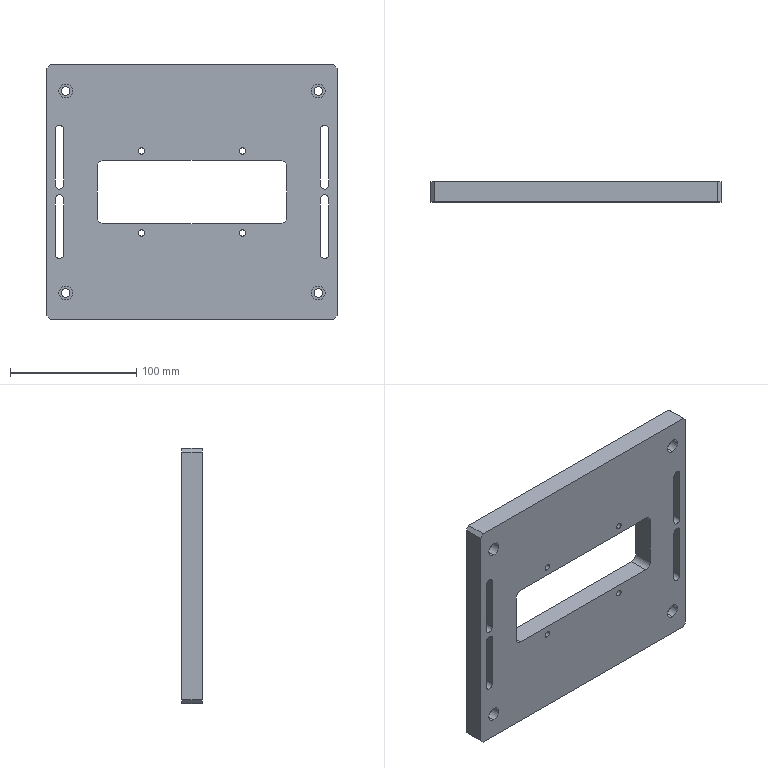Part | STEP file | 1 solid | 78 faces | box 230 x 16 x 202 mm | volume 593359 mm3 | cylinder 48 | plane 30 | commonest cylinder face diameters 6.5 x12 5 x8 6.6 x8 11 x8 20 x8 10 x4